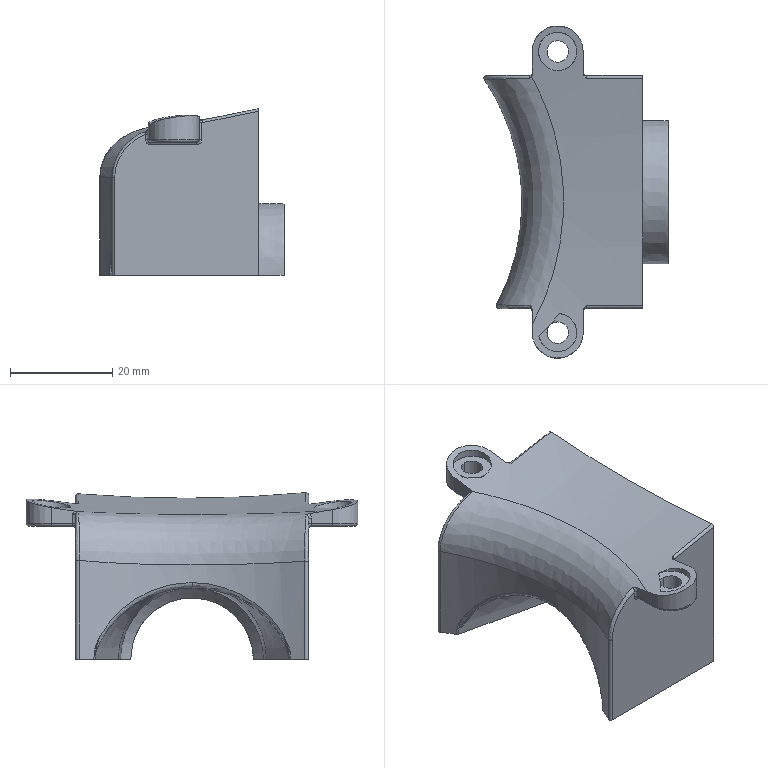Part | STEP file | ZXW722-L-50 | 1 solid | 111 faces | box 36.029 x 65 x 32.601 mm | volume 13339 mm3 | spline 44 | cylinder 28 | plane 18 | other 11 | torus 6 | sphere 4 | commonest cylinder face diameters 1 x16 4.2 x4 7.5 x2 10 x2 90.985 x2 85.985 x1